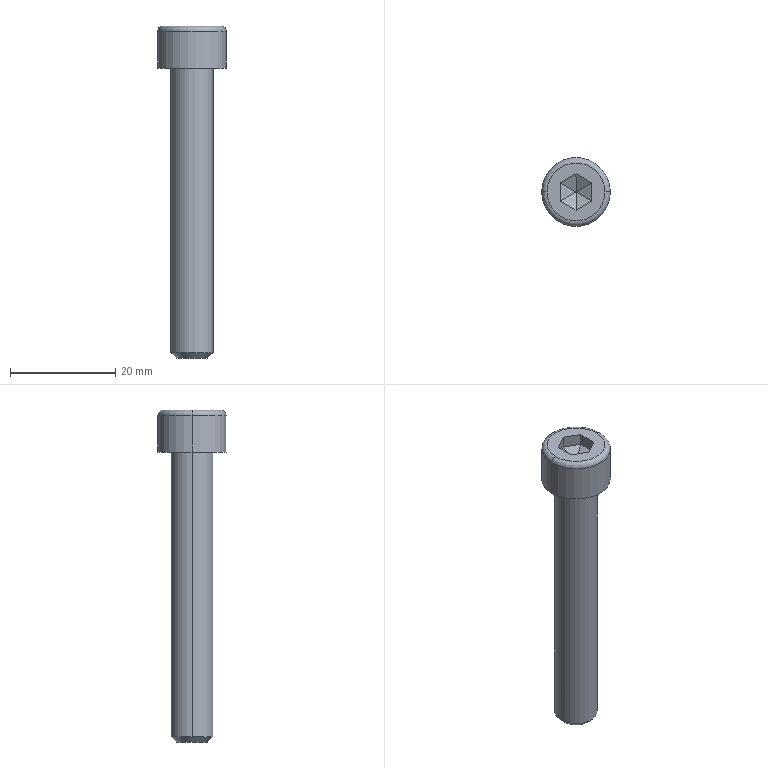Part | SolidWorks | features Chamfer 2, Fillet 2, ICE 2, Extrusion 1, RefAxis 1 | 1 solid | 26 faces | box 13 x 13 x 63 mm | volume 3718 mm3 | plane 16 | torus 4 | cylinder 4 | cone 2 | commonest cylinder face diameters 8 x2 13 x2
STEP:
#1=CARTESIAN_POINT('',(-4.1,0.,0.));
#2=VERTEX_POINT('',#1);
#3=CARTESIAN_POINT('',(4.1,0.,0.));
#4=VERTEX_POINT('',#3);
#5=CARTESIAN_POINT('',(0.,0.,0.));
#6=DIRECTION('',(0.,0.,1.));
#7=DIRECTION('',(1.,0.,0.));
#8=AXIS2_PLACEMENT_3D('',#5,#6,#7);
#9=CIRCLE('',#8,4.1);
#10=EDGE_CURVE('',#2,#4,#9,.T.);
#11=ORIENTED_EDGE('',*,*,#10,.F.);
#12=CARTESIAN_POINT('',(-4.,0.,-0.1));
#13=VERTEX_POINT('',#12);
#14=CARTESIAN_POINT('',(-4.1,0.,-0.1));
#15=DIRECTION('',(0.,1.,0.));
#16=DIRECTION('',(-1.,0.,0.));
#17=AXIS2_PLACEMENT_3D('',#14,#15,#16);
#18=CIRCLE('',#17,0.1);
#19=EDGE_CURVE('',#2,#13,#18,.T.);
#20=ORIENTED_EDGE('',*,*,#19,.T.);
#21=CARTESIAN_POINT('',(4.,0.,-0.1));
#22=VERTEX_POINT('',#21);
#23=CARTESIAN_POINT('',(0.,0.,-0.1));
#24=DIRECTION('',(0.,0.,-1.));
#25=DIRECTION('',(1.,0.,0.));
#26=AXIS2_PLACEMENT_3D('',#23,#24,#25);
#27=CIRCLE('',#26,4.);
#28=EDGE_CURVE('',#22,#13,#27,.T.);
#29=ORIENTED_EDGE('',*,*,#28,.F.);
#30=CARTESIAN_POINT('',(4.1,0.,-0.1));
#31=DIRECTION('',(0.,-1.,0.));
#32=DIRECTION('',(0.,0.,-1.));
#33=AXIS2_PLACEMENT_3D('',#30,#31,#32);
#34=CIRCLE('',#33,0.1);
#35=EDGE_CURVE('',#4,#22,#34,.T.);
#36=ORIENTED_EDGE('',*,*,#35,.F.);
#37=EDGE_LOOP('',(#11,#20,#29,#36));
#38=FACE_OUTER_BOUND('',#37,.T.);
#39=CARTESIAN_POINT('',(0.,0.,-0.1));
#40=DIRECTION('',(0.,0.,1.));
#41=DIRECTION('',(1.,0.,0.));
#42=AXIS2_PLACEMENT_3D('',#39,#40,#41);
#43=TOROIDAL_SURFACE('',#42,4.1,0.1);
#44=ADVANCED_FACE('',(#38),#43,.F.);
#45=CARTESIAN_POINT('',(-6.5,0.,7.));
#46=VERTEX_POINT('',#45);
#47=CARTESIAN_POINT('',(6.5,0.,7.));
#48=VERTEX_POINT('',#47);
#49=CARTESIAN_POINT('',(0.,0.,7.));
#50=DIRECTION('',(0.,0.,-1.));
#51=DIRECTION('',(1.,0.,0.));
#52=AXIS2_PLACEMENT_3D('',#49,#50,#51);
#53=CIRCLE('',#52,6.5);
#54=EDGE_CURVE('',#46,#48,#53,.T.);
#55=ORIENTED_EDGE('',*,*,#54,.F.);
#56=CARTESIAN_POINT('',(-5.5,0.,8.));
#57=VERTEX_POINT('',#56);
#58=CARTESIAN_POINT('',(-5.5,0.,7.));
#59=DIRECTION('',(0.,1.,0.));
#60=DIRECTION('',(-1.,0.,0.));
#61=AXIS2_PLACEMENT_3D('',#58,#59,#60);
#62=CIRCLE('',#61,1.);
#63=EDGE_CURVE('',#46,#57,#62,.T.);
#64=ORIENTED_EDGE('',*,*,#63,.T.);
#65=CARTESIAN_POINT('',(5.5,0.,8.));
#66=VERTEX_POINT('',#65);
#67=CARTESIAN_POINT('',(0.,0.,8.));
#68=DIRECTION('',(0.,0.,1.));
#69=DIRECTION('',(1.,0.,0.));
#70=AXIS2_PLACEMENT_3D('',#67,#68,#69);
#71=CIRCLE('',#70,5.5);
#72=EDGE_CURVE('',#66,#57,#71,.T.);
#73=ORIENTED_EDGE('',*,*,#72,.F.);
#74=CARTESIAN_POINT('',(5.5,0.,7.));
#75=DIRECTION('',(0.,-1.,0.));
#76=DIRECTION('',(0.,0.,-1.));
#77=AXIS2_PLACEMENT_3D('',#74,#75,#76);
#78=CIRCLE('',#77,1.);
#79=EDGE_CURVE('',#48,#66,#78,.T.);
#80=ORIENTED_EDGE('',*,*,#79,.F.);
#81=EDGE_LOOP('',(#55,#64,#73,#80));
#82=FACE_OUTER_BOUND('',#81,.T.);
#83=CARTESIAN_POINT('',(0.,0.,7.));
#84=DIRECTION('',(0.,0.,1.));
#85=DIRECTION('',(1.,0.,0.));
#86=AXIS2_PLACEMENT_3D('',#83,#84,#85);
#87=TOROIDAL_SURFACE('',#86,5.5,1.);
#88=ADVANCED_FACE('',(#82),#87,.T.);
#89=CARTESIAN_POINT('',(-3.,0.,-55.));
#90=VERTEX_POINT('',#89);
#91=CARTESIAN_POINT('',(3.,0.,-55.));
#92=VERTEX_POINT('',#91);
#93=CARTESIAN_POINT('',(0.,0.,-55.));
#94=DIRECTION('',(0.,0.,-1.));
#95=DIRECTION('',(-1.,0.,0.));
#96=AXIS2_PLACEMENT_3D('',#93,#94,#95);
#97=CIRCLE('',#96,3.);
#98=EDGE_CURVE('',#90,#92,#97,.T.);
#99=ORIENTED_EDGE('',*,*,#98,.F.);
#100=CARTESIAN_POINT('',(-4.,0.,-54.));
#101=VERTEX_POINT('',#100);
#102=CARTESIAN_POINT('',(-3.,0.,-55.));
#103=DIRECTION('',(-0.7071,0.,0.7071));
#104=VECTOR('',#103,1000.);
#105=LINE('',#102,#104);
#106=EDGE_CURVE('',#90,#101,#105,.T.);
#107=ORIENTED_EDGE('',*,*,#106,.T.);
#108=CARTESIAN_POINT('',(4.,0.,-54.));
#109=VERTEX_POINT('',#108);
#110=CARTESIAN_POINT('',(0.,0.,-54.));
#111=DIRECTION('',(0.,0.,1.));
#112=DIRECTION('',(-1.,0.,0.));
#113=AXIS2_PLACEMENT_3D('',#110,#111,#112);
#114=CIRCLE('',#113,4.);
#115=EDGE_CURVE('',#109,#101,#114,.T.);
#116=ORIENTED_EDGE('',*,*,#115,.F.);
#117=CARTESIAN_POINT('',(3.,0.,-55.));
#118=DIRECTION('',(0.7071,0.,0.7071));
#119=VECTOR('',#118,1000.);
#120=LINE('',#117,#119);
#121=EDGE_CURVE('',#92,#109,#120,.T.);
#122=ORIENTED_EDGE('',*,*,#121,.F.);
#123=EDGE_LOOP('',(#99,#107,#116,#122));
#124=FACE_OUTER_BOUND('',#123,.T.);
#125=CARTESIAN_POINT('',(0.,0.,-55.));
#126=DIRECTION('',(0.,0.,1.));
#127=DIRECTION('',(1.,0.,0.));
#128=AXIS2_PLACEMENT_3D('',#125,#126,#127);
#129=CONICAL_SURFACE('',#128,3.,0.7854);
#130=ADVANCED_FACE('',(#124),#129,.T.);
#131=ORIENTED_EDGE('',*,*,#115,.T.);
#132=CARTESIAN_POINT('',(-4.,0.,-55.));
#133=DIRECTION('',(0.,0.,1.));
#134=VECTOR('',#133,1000.);
#135=LINE('',#132,#134);
#136=EDGE_CURVE('',#101,#13,#135,.T.);
#137=ORIENTED_EDGE('',*,*,#136,.T.);
#138=CARTESIAN_POINT('',(0.,0.,-0.1));
#139=DIRECTION('',(0.,0.,-1.));
#140=DIRECTION('',(1.,0.,0.));
#141=AXIS2_PLACEMENT_3D('',#138,#139,#140);
#142=CIRCLE('',#141,4.);
#143=EDGE_CURVE('',#13,#22,#142,.T.);
#144=ORIENTED_EDGE('',*,*,#143,.T.);
#145=CARTESIAN_POINT('',(4.,0.,-55.));
#146=DIRECTION('',(0.,0.,1.));
#147=VECTOR('',#146,1000.);
#148=LINE('',#145,#147);
#149=EDGE_CURVE('',#109,#22,#148,.T.);
#150=ORIENTED_EDGE('',*,*,#149,.F.);
#151=EDGE_LOOP('',(#131,#137,#144,#150));
#152=FACE_OUTER_BOUND('',#151,.T.);
#153=CARTESIAN_POINT('',(0.,0.,-55.));
#154=DIRECTION('',(0.,0.,1.));
#155=DIRECTION('',(1.,0.,0.));
#156=AXIS2_PLACEMENT_3D('',#153,#154,#155);
#157=CYLINDRICAL_SURFACE('',#156,4.);
#158=ADVANCED_FACE('',(#152),#157,.T.);
#159=ORIENTED_EDGE('',*,*,#54,.T.);
#160=CARTESIAN_POINT('',(6.5,0.,0.));
#161=VERTEX_POINT('',#160);
#162=CARTESIAN_POINT('',(6.5,0.,8.));
#163=DIRECTION('',(0.,0.,-1.));
#164=VECTOR('',#163,1000.);
#165=LINE('',#162,#164);
#166=EDGE_CURVE('',#48,#161,#165,.T.);
#167=ORIENTED_EDGE('',*,*,#166,.T.);
#168=CARTESIAN_POINT('',(-6.5,0.,0.));
#169=VERTEX_POINT('',#168);
#170=CARTESIAN_POINT('',(0.,0.,0.));
#171=DIRECTION('',(0.,0.,1.));
#172=DIRECTION('',(1.,0.,0.));
#173=AXIS2_PLACEMENT_3D('',#170,#171,#172);
#174=CIRCLE('',#173,6.5);
#175=EDGE_CURVE('',#161,#169,#174,.T.);
#176=ORIENTED_EDGE('',*,*,#175,.T.);
#177=CARTESIAN_POINT('',(-6.5,0.,8.));
#178=DIRECTION('',(0.,0.,-1.));
#179=VECTOR('',#178,1000.);
#180=LINE('',#177,#179);
#181=EDGE_CURVE('',#46,#169,#180,.T.);
#182=ORIENTED_EDGE('',*,*,#181,.F.);
#183=EDGE_LOOP('',(#159,#167,#176,#182));
#184=FACE_OUTER_BOUND('',#183,.T.);
#185=CARTESIAN_POINT('',(0.,0.,8.));
#186=DIRECTION('',(0.,0.,-1.));
#187=DIRECTION('',(-1.,0.,0.));
#188=AXIS2_PLACEMENT_3D('',#185,#186,#187);
#189=CYLINDRICAL_SURFACE('',#188,6.5);
#190=ADVANCED_FACE('',(#184),#189,.T.);
#191=CARTESIAN_POINT('',(0.,0.,0.));
#192=DIRECTION('',(0.,0.,1.));
#193=DIRECTION('',(1.,0.,0.));
#194=AXIS2_PLACEMENT_3D('',#191,#192,#193);
#195=CIRCLE('',#194,4.1);
#196=EDGE_CURVE('',#4,#2,#195,.T.);
#197=ORIENTED_EDGE('',*,*,#196,.T.);
#198=ORIENTED_EDGE('',*,*,#10,.T.);
#199=EDGE_LOOP('',(#197,#198));
#200=FACE_BOUND('',#199,.T.);
#201=CARTESIAN_POINT('',(0.,0.,0.));
#202=DIRECTION('',(0.,0.,1.));
#203=DIRECTION('',(1.,0.,0.));
#204=AXIS2_PLACEMENT_3D('',#201,#202,#203);
#205=CIRCLE('',#204,6.5);
#206=EDGE_CURVE('',#169,#161,#205,.T.);
#207=ORIENTED_EDGE('',*,*,#206,.F.);
#208=ORIENTED_EDGE('',*,*,#175,.F.);
#209=EDGE_LOOP('',(#207,#208));
#210=FACE_OUTER_BOUND('',#209,.T.);
#211=CARTESIAN_POINT('',(0.,0.,0.));
#212=DIRECTION('',(0.,0.,1.));
#213=DIRECTION('',(1.,0.,0.));
#214=AXIS2_PLACEMENT_3D('',#211,#212,#213);
#215=PLANE('',#214);
#216=ADVANCED_FACE('',(#200,#210),#215,.F.);
#217=ORIENTED_EDGE('',*,*,#166,.F.);
#218=CARTESIAN_POINT('',(0.,0.,7.));
#219=DIRECTION('',(0.,0.,-1.));
#220=DIRECTION('',(1.,0.,0.));
#221=AXIS2_PLACEMENT_3D('',#218,#219,#220);
#222=CIRCLE('',#221,6.5);
#223=EDGE_CURVE('',#48,#46,#222,.T.);
#224=ORIENTED_EDGE('',*,*,#223,.T.);
#225=ORIENTED_EDGE('',*,*,#181,.T.);
#226=ORIENTED_EDGE('',*,*,#206,.T.);
#227=EDGE_LOOP('',(#217,#224,#225,#226));
#228=FACE_OUTER_BOUND('',#227,.T.);
#229=CARTESIAN_POINT('',(0.,0.,8.));
#230=DIRECTION('',(0.,0.,-1.));
#231=DIRECTION('',(-1.,0.,0.));
#232=AXIS2_PLACEMENT_3D('',#229,#230,#231);
#233=CYLINDRICAL_SURFACE('',#232,6.5);
#234=ADVANCED_FACE('',(#228),#233,.T.);
#235=ORIENTED_EDGE('',*,*,#72,.T.);
#236=CARTESIAN_POINT('',(0.,0.,8.));
#237=DIRECTION('',(0.,0.,1.));
#238=DIRECTION('',(1.,0.,0.));
#239=AXIS2_PLACEMENT_3D('',#236,#237,#238);
#240=CIRCLE('',#239,5.5);
#241=EDGE_CURVE('',#57,#66,#240,.T.);
#242=ORIENTED_EDGE('',*,*,#241,.T.);
#243=EDGE_LOOP('',(#235,#242));
#244=FACE_OUTER_BOUND('',#243,.T.);
#245=CARTESIAN_POINT('',(3.,-1.732,8.));
#246=VERTEX_POINT('',#245);
#247=CARTESIAN_POINT('',(3.,1.732,8.));
#248=VERTEX_POINT('',#247);
#249=CARTESIAN_POINT('',(3.,-1.732,8.));
#250=DIRECTION('',(0.,1.,0.));
#251=VECTOR('',#250,1000.);
#252=LINE('',#249,#251);
#253=EDGE_CURVE('',#246,#248,#252,.T.);
#254=ORIENTED_EDGE('',*,*,#253,.F.);
#255=CARTESIAN_POINT('',(0.,-3.464,8.));
#256=VERTEX_POINT('',#255);
#257=CARTESIAN_POINT('',(0.,-3.464,8.));
#258=DIRECTION('',(0.866,0.5,0.));
#259=VECTOR('',#258,1000.);
#260=LINE('',#257,#259);
#261=EDGE_CURVE('',#256,#246,#260,.T.);
#262=ORIENTED_EDGE('',*,*,#261,.F.);
#263=CARTESIAN_POINT('',(-3.,-1.732,8.));
#264=VERTEX_POINT('',#263);
#265=CARTESIAN_POINT('',(-3.,-1.732,8.));
#266=DIRECTION('',(0.866,-0.5,0.));
#267=VECTOR('',#266,1000.);
#268=LINE('',#265,#267);
#269=EDGE_CURVE('',#264,#256,#268,.T.);
#270=ORIENTED_EDGE('',*,*,#269,.F.);
#271=CARTESIAN_POINT('',(-3.,1.732,8.));
#272=VERTEX_POINT('',#271);
#273=CARTESIAN_POINT('',(-3.,1.732,8.));
#274=DIRECTION('',(0.,-1.,0.));
#275=VECTOR('',#274,1000.);
#276=LINE('',#273,#275);
#277=EDGE_CURVE('',#272,#264,#276,.T.);
#278=ORIENTED_EDGE('',*,*,#277,.F.);
#279=CARTESIAN_POINT('',(0.,3.464,8.));
#280=VERTEX_POINT('',#279);
#281=CARTESIAN_POINT('',(0.,3.464,8.));
#282=DIRECTION('',(-0.866,-0.5,0.));
#283=VECTOR('',#282,1000.);
#284=LINE('',#281,#283);
#285=EDGE_CURVE('',#280,#272,#284,.T.);
#286=ORIENTED_EDGE('',*,*,#285,.F.);
#287=CARTESIAN_POINT('',(3.,1.732,8.));
#288=DIRECTION('',(-0.866,0.5,0.));
#289=VECTOR('',#288,1000.);
#290=LINE('',#287,#289);
#291=EDGE_CURVE('',#248,#280,#290,.T.);
#292=ORIENTED_EDGE('',*,*,#291,.F.);
#293=EDGE_LOOP('',(#254,#262,#270,#278,#286,#292));
#294=FACE_BOUND('',#293,.T.);
#295=CARTESIAN_POINT('',(0.,0.,8.));
#296=DIRECTION('',(0.,0.,1.));
#297=DIRECTION('',(1.,0.,0.));
#298=AXIS2_PLACEMENT_3D('',#295,#296,#297);
#299=PLANE('',#298);
#300=ADVANCED_FACE('',(#244,#294),#299,.T.);
#301=CARTESIAN_POINT('',(3.,1.732,5.729));
#302=VERTEX_POINT('',#301);
#303=CARTESIAN_POINT('',(3.,1.732,4.));
#304=DIRECTION('',(0.,0.,1.));
#305=VECTOR('',#304,1000.);
#306=LINE('',#303,#305);
#307=EDGE_CURVE('',#302,#248,#306,.T.);
#308=ORIENTED_EDGE('',*,*,#307,.F.);
#309=CARTESIAN_POINT('',(3.,-1.732,5.729));
#310=VERTEX_POINT('',#309);
#311=CARTESIAN_POINT('',(3.,-1.732,5.729));
#312=DIRECTION('',(0.,-1.,0.));
#313=VECTOR('',#312,1000.);
#314=LINE('',#311,#313);
#315=EDGE_CURVE('',#302,#310,#314,.T.);
#316=ORIENTED_EDGE('',*,*,#315,.T.);
#317=CARTESIAN_POINT('',(3.,-1.732,4.));
#318=DIRECTION('',(0.,0.,1.));
#319=VECTOR('',#318,1000.);
#320=LINE('',#317,#319);
#321=EDGE_CURVE('',#310,#246,#320,.T.);
#322=ORIENTED_EDGE('',*,*,#321,.T.);
#323=ORIENTED_EDGE('',*,*,#253,.T.);
#324=EDGE_LOOP('',(#308,#316,#322,#323));
#325=FACE_OUTER_BOUND('',#324,.T.);
#326=CARTESIAN_POINT('',(3.,-1.732,4.));
#327=DIRECTION('',(1.,0.,0.));
#328=DIRECTION('',(0.,1.,0.));
#329=AXIS2_PLACEMENT_3D('',#326,#327,#328);
#330=PLANE('',#329);
#331=ADVANCED_FACE('',(#325),#330,.F.);
#332=ORIENTED_EDGE('',*,*,#321,.F.);
#333=CARTESIAN_POINT('',(0.,-3.464,5.729));
#334=VERTEX_POINT('',#333);
#335=CARTESIAN_POINT('',(0.,-3.464,5.729));
#336=DIRECTION('',(-0.866,-0.5,0.));
#337=VECTOR('',#336,1000.);
#338=LINE('',#335,#337);
#339=EDGE_CURVE('',#310,#334,#338,.T.);
#340=ORIENTED_EDGE('',*,*,#339,.T.);
#341=CARTESIAN_POINT('',(0.,-3.464,4.));
#342=DIRECTION('',(0.,0.,1.));
#343=VECTOR('',#342,1000.);
#344=LINE('',#341,#343);
#345=EDGE_CURVE('',#334,#256,#344,.T.);
#346=ORIENTED_EDGE('',*,*,#345,.T.);
#347=ORIENTED_EDGE('',*,*,#261,.T.);
#348=EDGE_LOOP('',(#332,#340,#346,#347));
#349=FACE_OUTER_BOUND('',#348,.T.);
#350=CARTESIAN_POINT('',(0.,-3.464,4.));
#351=DIRECTION('',(0.5,-0.866,0.));
#352=DIRECTION('',(0.866,0.5,0.));
#353=AXIS2_PLACEMENT_3D('',#350,#351,#352);
#354=PLANE('',#353);
#355=ADVANCED_FACE('',(#349),#354,.F.);
#356=ORIENTED_EDGE('',*,*,#345,.F.);
#357=CARTESIAN_POINT('',(-3.,-1.732,5.729));
#358=VERTEX_POINT('',#357);
#359=CARTESIAN_POINT('',(-3.,-1.732,5.729));
#360=DIRECTION('',(-0.866,0.5,0.));
#361=VECTOR('',#360,1000.);
#362=LINE('',#359,#361);
#363=EDGE_CURVE('',#334,#358,#362,.T.);
#364=ORIENTED_EDGE('',*,*,#363,.T.);
#365=CARTESIAN_POINT('',(-3.,-1.732,4.));
#366=DIRECTION('',(0.,0.,1.));
#367=VECTOR('',#366,1000.);
#368=LINE('',#365,#367);
#369=EDGE_CURVE('',#358,#264,#368,.T.);
#370=ORIENTED_EDGE('',*,*,#369,.T.);
#371=ORIENTED_EDGE('',*,*,#269,.T.);
#372=EDGE_LOOP('',(#356,#364,#370,#371));
#373=FACE_OUTER_BOUND('',#372,.T.);
#374=CARTESIAN_POINT('',(-3.,-1.732,4.));
#375=DIRECTION('',(-0.5,-0.866,0.));
#376=DIRECTION('',(0.866,-0.5,0.));
#377=AXIS2_PLACEMENT_3D('',#374,#375,#376);
#378=PLANE('',#377);
#379=ADVANCED_FACE('',(#373),#378,.F.);
#380=ORIENTED_EDGE('',*,*,#369,.F.);
#381=CARTESIAN_POINT('',(-3.,1.732,5.729));
#382=VERTEX_POINT('',#381);
#383=CARTESIAN_POINT('',(-3.,1.732,5.729));
#384=DIRECTION('',(0.,1.,0.));
#385=VECTOR('',#384,1000.);
#386=LINE('',#383,#385);
#387=EDGE_CURVE('',#358,#382,#386,.T.);
#388=ORIENTED_EDGE('',*,*,#387,.T.);
#389=CARTESIAN_POINT('',(-3.,1.732,4.));
#390=DIRECTION('',(0.,0.,1.));
#391=VECTOR('',#390,1000.);
#392=LINE('',#389,#391);
#393=EDGE_CURVE('',#382,#272,#392,.T.);
#394=ORIENTED_EDGE('',*,*,#393,.T.);
#395=ORIENTED_EDGE('',*,*,#277,.T.);
#396=EDGE_LOOP('',(#380,#388,#394,#395));
#397=FACE_OUTER_BOUND('',#396,.T.);
#398=CARTESIAN_POINT('',(-3.,1.732,4.));
#399=DIRECTION('',(-1.,0.,0.));
#400=DIRECTION('',(0.,0.,1.));
#401=AXIS2_PLACEMENT_3D('',#398,#399,#400);
#402=PLANE('',#401);
#403=ADVANCED_FACE('',(#397),#402,.F.);
#404=ORIENTED_EDGE('',*,*,#393,.F.);
#405=CARTESIAN_POINT('',(0.,3.464,5.729));
#406=VERTEX_POINT('',#405);
#407=CARTESIAN_POINT('',(0.,3.464,5.729));
#408=DIRECTION('',(0.866,0.5,0.));
#409=VECTOR('',#408,1000.);
#410=LINE('',#407,#409);
#411=EDGE_CURVE('',#382,#406,#410,.T.);
#412=ORIENTED_EDGE('',*,*,#411,.T.);
#413=CARTESIAN_POINT('',(0.,3.464,4.));
#414=DIRECTION('',(0.,0.,1.));
#415=VECTOR('',#414,1000.);
#416=LINE('',#413,#415);
#417=EDGE_CURVE('',#406,#280,#416,.T.);
#418=ORIENTED_EDGE('',*,*,#417,.T.);
#419=ORIENTED_EDGE('',*,*,#285,.T.);
#420=EDGE_LOOP('',(#404,#412,#418,#419));
#421=FACE_OUTER_BOUND('',#420,.T.);
#422=CARTESIAN_POINT('',(0.,3.464,4.));
#423=DIRECTION('',(-0.5,0.866,0.));
#424=DIRECTION('',(-0.866,-0.5,0.));
#425=AXIS2_PLACEMENT_3D('',#422,#423,#424);
#426=PLANE('',#425);
#427=ADVANCED_FACE('',(#421),#426,.F.);
#428=ORIENTED_EDGE('',*,*,#417,.F.);
#429=CARTESIAN_POINT('',(3.,1.732,5.729));
#430=DIRECTION('',(0.866,-0.5,0.));
#431=VECTOR('',#430,1000.);
#432=LINE('',#429,#431);
#433=EDGE_CURVE('',#406,#302,#432,.T.);
#434=ORIENTED_EDGE('',*,*,#433,.T.);
#435=ORIENTED_EDGE('',*,*,#307,.T.);
#436=ORIENTED_EDGE('',*,*,#291,.T.);
#437=EDGE_LOOP('',(#428,#434,#435,#436));
#438=FACE_OUTER_BOUND('',#437,.T.);
#439=CARTESIAN_POINT('',(3.,1.732,4.));
#440=DIRECTION('',(0.5,0.866,0.));
#441=DIRECTION('',(-0.866,0.5,0.));
#442=AXIS2_PLACEMENT_3D('',#439,#440,#441);
#443=PLANE('',#442);
#444=ADVANCED_FACE('',(#438),#443,.F.);
#445=CARTESIAN_POINT('',(0.,0.005888,4.));
#446=VERTEX_POINT('',#445);
#447=CARTESIAN_POINT('',(-0.005099,0.002944,4.));
#448=VERTEX_POINT('',#447);
#449=CARTESIAN_POINT('',(-0.00255,0.004416,4.));
#450=DIRECTION('',(-0.866,-0.5,0.));
#451=VECTOR('',#450,1000.);
#452=LINE('',#449,#451);
#453=EDGE_CURVE('',#446,#448,#452,.T.);
#454=ORIENTED_EDGE('',*,*,#453,.T.);
#455=CARTESIAN_POINT('',(-0.005099,-0.002944,4.));
#456=VERTEX_POINT('',#455);
#457=CARTESIAN_POINT('',(-0.005099,0.,4.));
#458=DIRECTION('',(0.,-1.,0.));
#459=VECTOR('',#458,1000.);
#460=LINE('',#457,#459);
#461=EDGE_CURVE('',#448,#456,#460,.T.);
#462=ORIENTED_EDGE('',*,*,#461,.T.);
#463=CARTESIAN_POINT('',(0.,-0.005888,4.));
#464=VERTEX_POINT('',#463);
#465=CARTESIAN_POINT('',(-0.00255,-0.004416,4.));
#466=DIRECTION('',(0.866,-0.5,0.));
#467=VECTOR('',#466,1000.);
#468=LINE('',#465,#467);
#469=EDGE_CURVE('',#456,#464,#468,.T.);
#470=ORIENTED_EDGE('',*,*,#469,.T.);
#471=CARTESIAN_POINT('',(0.005099,-0.002944,4.));
#472=VERTEX_POINT('',#471);
#473=CARTESIAN_POINT('',(0.00255,-0.004416,4.));
#474=DIRECTION('',(0.866,0.5,0.));
#475=VECTOR('',#474,1000.);
#476=LINE('',#473,#475);
#477=EDGE_CURVE('',#464,#472,#476,.T.);
#478=ORIENTED_EDGE('',*,*,#477,.T.);
#479=CARTESIAN_POINT('',(0.005099,0.002944,4.));
#480=VERTEX_POINT('',#479);
#481=CARTESIAN_POINT('',(0.005099,0.,4.));
#482=DIRECTION('',(0.,1.,0.));
#483=VECTOR('',#482,1000.);
#484=LINE('',#481,#483);
#485=EDGE_CURVE('',#472,#480,#484,.T.);
#486=ORIENTED_EDGE('',*,*,#485,.T.);
#487=CARTESIAN_POINT('',(0.00255,0.004416,4.));
#488=DIRECTION('',(-0.866,0.5,0.));
#489=VECTOR('',#488,1000.);
#490=LINE('',#487,#489);
#491=EDGE_CURVE('',#480,#446,#490,.T.);
#492=ORIENTED_EDGE('',*,*,#491,.T.);
#493=EDGE_LOOP('',(#454,#462,#470,#478,#486,#492));
#494=FACE_OUTER_BOUND('',#493,.T.);
#495=CARTESIAN_POINT('',(0.,0.,4.));
#496=DIRECTION('',(0.,0.,1.));
#497=DIRECTION('',(1.,0.,0.));
#498=AXIS2_PLACEMENT_3D('',#495,#496,#497);
#499=PLANE('',#498);
#500=ADVANCED_FACE('',(#494),#499,.T.);
#501=ORIENTED_EDGE('',*,*,#136,.F.);
#502=CARTESIAN_POINT('',(0.,0.,-54.));
#503=DIRECTION('',(0.,0.,1.));
#504=DIRECTION('',(-1.,0.,0.));
#505=AXIS2_PLACEMENT_3D('',#502,#503,#504);
#506=CIRCLE('',#505,4.);
#507=EDGE_CURVE('',#101,#109,#506,.T.);
#508=ORIENTED_EDGE('',*,*,#507,.T.);
#509=ORIENTED_EDGE('',*,*,#149,.T.);
#510=ORIENTED_EDGE('',*,*,#28,.T.);
#511=EDGE_LOOP('',(#501,#508,#509,#510));
#512=FACE_OUTER_BOUND('',#511,.T.);
#513=CARTESIAN_POINT('',(0.,0.,-55.));
#514=DIRECTION('',(0.,0.,1.));
#515=DIRECTION('',(1.,0.,0.));
#516=AXIS2_PLACEMENT_3D('',#513,#514,#515);
#517=CYLINDRICAL_SURFACE('',#516,4.);
#518=ADVANCED_FACE('',(#512),#517,.T.);
#519=CARTESIAN_POINT('',(0.,0.,-55.));
#520=DIRECTION('',(0.,0.,-1.));
#521=DIRECTION('',(-1.,0.,0.));
#522=AXIS2_PLACEMENT_3D('',#519,#520,#521);
#523=CIRCLE('',#522,3.);
#524=EDGE_CURVE('',#92,#90,#523,.T.);
#525=ORIENTED_EDGE('',*,*,#524,.T.);
#526=ORIENTED_EDGE('',*,*,#98,.T.);
#527=EDGE_LOOP('',(#525,#526));
#528=FACE_OUTER_BOUND('',#527,.T.);
#529=CARTESIAN_POINT('',(0.,0.,-55.));
#530=DIRECTION('',(0.,0.,-1.));
#531=DIRECTION('',(-1.,0.,0.));
#532=AXIS2_PLACEMENT_3D('',#529,#530,#531);
#533=PLANE('',#532);
#534=ADVANCED_FACE('',(#528),#533,.T.);
#535=ORIENTED_EDGE('',*,*,#106,.F.);
#536=ORIENTED_EDGE('',*,*,#524,.F.);
#537=ORIENTED_EDGE('',*,*,#121,.T.);
#538=ORIENTED_EDGE('',*,*,#507,.F.);
#539=EDGE_LOOP('',(#535,#536,#537,#538));
#540=FACE_OUTER_BOUND('',#539,.T.);
#541=CARTESIAN_POINT('',(0.,0.,-55.));
#542=DIRECTION('',(0.,0.,1.));
#543=DIRECTION('',(1.,0.,0.));
#544=AXIS2_PLACEMENT_3D('',#541,#542,#543);
#545=CONICAL_SURFACE('',#544,3.,0.7854);
#546=ADVANCED_FACE('',(#540),#545,.T.);
#547=ORIENTED_EDGE('',*,*,#63,.F.);
#548=ORIENTED_EDGE('',*,*,#223,.F.);
#549=ORIENTED_EDGE('',*,*,#79,.T.);
#550=ORIENTED_EDGE('',*,*,#241,.F.);
#551=EDGE_LOOP('',(#547,#548,#549,#550));
#552=FACE_OUTER_BOUND('',#551,.T.);
#553=CARTESIAN_POINT('',(0.,0.,7.));
#554=DIRECTION('',(0.,0.,1.));
#555=DIRECTION('',(1.,0.,0.));
#556=AXIS2_PLACEMENT_3D('',#553,#554,#555);
#557=TOROIDAL_SURFACE('',#556,5.5,1.);
#558=ADVANCED_FACE('',(#552),#557,.T.);
#559=CARTESIAN_POINT('',(0.00408,-0.002355,3.999));
#560=DIRECTION('',(-0.7746,0.4472,-0.4472));
#561=VECTOR('',#560,1000.);
#562=LINE('',#559,#561);
#563=EDGE_CURVE('',#310,#472,#562,.T.);
#564=ORIENTED_EDGE('',*,*,#563,.F.);
#565=ORIENTED_EDGE('',*,*,#315,.F.);
#566=CARTESIAN_POINT('',(0.00408,0.002355,3.999));
#567=DIRECTION('',(0.7746,0.4472,0.4472));
#568=VECTOR('',#567,1000.);
#569=LINE('',#566,#568);
#570=EDGE_CURVE('',#480,#302,#569,.T.);
#571=ORIENTED_EDGE('',*,*,#570,.F.);
#572=ORIENTED_EDGE('',*,*,#485,.F.);
#573=EDGE_LOOP('',(#564,#565,#571,#572));
#574=FACE_OUTER_BOUND('',#573,.T.);
#575=CARTESIAN_POINT('',(0.005099,0.,4.));
#576=DIRECTION('',(0.5,0.,-0.866));
#577=DIRECTION('',(0.,1.,0.));
#578=AXIS2_PLACEMENT_3D('',#575,#576,#577);
#579=PLANE('',#578);
#580=ADVANCED_FACE('',(#574),#579,.F.);
#581=ORIENTED_EDGE('',*,*,#570,.T.);
#582=ORIENTED_EDGE('',*,*,#433,.F.);
#583=CARTESIAN_POINT('',(0.,0.004711,3.999));
#584=DIRECTION('',(0.,0.8944,0.4472));
#585=VECTOR('',#584,1000.);
#586=LINE('',#583,#585);
#587=EDGE_CURVE('',#446,#406,#586,.T.);
#588=ORIENTED_EDGE('',*,*,#587,.F.);
#589=ORIENTED_EDGE('',*,*,#491,.F.);
#590=EDGE_LOOP('',(#581,#582,#588,#589));
#591=FACE_OUTER_BOUND('',#590,.T.);
#592=CARTESIAN_POINT('',(0.00255,0.004416,4.));
#593=DIRECTION('',(0.25,0.433,-0.866));
#594=DIRECTION('',(-0.866,0.5,0.));
#595=AXIS2_PLACEMENT_3D('',#592,#593,#594);
#596=PLANE('',#595);
#597=ADVANCED_FACE('',(#591),#596,.F.);
#598=ORIENTED_EDGE('',*,*,#563,.T.);
#599=ORIENTED_EDGE('',*,*,#477,.F.);
#600=CARTESIAN_POINT('',(0.,-0.004711,3.999));
#601=DIRECTION('',(0.,0.8944,-0.4472));
#602=VECTOR('',#601,1000.);
#603=LINE('',#600,#602);
#604=EDGE_CURVE('',#334,#464,#603,.T.);
#605=ORIENTED_EDGE('',*,*,#604,.F.);
#606=ORIENTED_EDGE('',*,*,#339,.F.);
#607=EDGE_LOOP('',(#598,#599,#605,#606));
#608=FACE_OUTER_BOUND('',#607,.T.);
#609=CARTESIAN_POINT('',(0.00255,-0.004416,4.));
#610=DIRECTION('',(0.25,-0.433,-0.866));
#611=DIRECTION('',(0.866,0.5,0.));
#612=AXIS2_PLACEMENT_3D('',#609,#610,#611);
#613=PLANE('',#612);
#614=ADVANCED_FACE('',(#608),#613,.F.);
#615=ORIENTED_EDGE('',*,*,#587,.T.);
#616=ORIENTED_EDGE('',*,*,#411,.F.);
#617=CARTESIAN_POINT('',(-0.00408,0.002355,3.999));
#618=DIRECTION('',(-0.7746,0.4472,0.4472));
#619=VECTOR('',#618,1000.);
#620=LINE('',#617,#619);
#621=EDGE_CURVE('',#448,#382,#620,.T.);
#622=ORIENTED_EDGE('',*,*,#621,.F.);
#623=ORIENTED_EDGE('',*,*,#453,.F.);
#624=EDGE_LOOP('',(#615,#616,#622,#623));
#625=FACE_OUTER_BOUND('',#624,.T.);
#626=CARTESIAN_POINT('',(-0.00255,0.004416,4.));
#627=DIRECTION('',(-0.25,0.433,-0.866));
#628=DIRECTION('',(-0.866,-0.5,0.));
#629=AXIS2_PLACEMENT_3D('',#626,#627,#628);
#630=PLANE('',#629);
#631=ADVANCED_FACE('',(#625),#630,.F.);
#632=ORIENTED_EDGE('',*,*,#604,.T.);
#633=ORIENTED_EDGE('',*,*,#469,.F.);
#634=CARTESIAN_POINT('',(-0.00408,-0.002355,3.999));
#635=DIRECTION('',(0.7746,0.4472,-0.4472));
#636=VECTOR('',#635,1000.);
#637=LINE('',#634,#636);
#638=EDGE_CURVE('',#358,#456,#637,.T.);
#639=ORIENTED_EDGE('',*,*,#638,.F.);
#640=ORIENTED_EDGE('',*,*,#363,.F.);
#641=EDGE_LOOP('',(#632,#633,#639,#640));
#642=FACE_OUTER_BOUND('',#641,.T.);
#643=CARTESIAN_POINT('',(-0.00255,-0.004416,4.));
#644=DIRECTION('',(-0.25,-0.433,-0.866));
#645=DIRECTION('',(0.866,-0.5,0.));
#646=AXIS2_PLACEMENT_3D('',#643,#644,#645);
#647=PLANE('',#646);
#648=ADVANCED_FACE('',(#642),#647,.F.);
#649=ORIENTED_EDGE('',*,*,#621,.T.);
#650=ORIENTED_EDGE('',*,*,#387,.F.);
#651=ORIENTED_EDGE('',*,*,#638,.T.);
#652=ORIENTED_EDGE('',*,*,#461,.F.);
#653=EDGE_LOOP('',(#649,#650,#651,#652));
#654=FACE_OUTER_BOUND('',#653,.T.);
#655=CARTESIAN_POINT('',(-0.005099,0.,4.));
#656=DIRECTION('',(-0.5,0.,-0.866));
#657=DIRECTION('',(0.,-1.,0.));
#658=AXIS2_PLACEMENT_3D('',#655,#656,#657);
#659=PLANE('',#658);
#660=ADVANCED_FACE('',(#654),#659,.F.);
#661=ORIENTED_EDGE('',*,*,#19,.F.);
#662=ORIENTED_EDGE('',*,*,#196,.F.);
#663=ORIENTED_EDGE('',*,*,#35,.T.);
#664=ORIENTED_EDGE('',*,*,#143,.F.);
#665=EDGE_LOOP('',(#661,#662,#663,#664));
#666=FACE_OUTER_BOUND('',#665,.T.);
#667=CARTESIAN_POINT('',(0.,0.,-0.1));
#668=DIRECTION('',(0.,0.,1.));
#669=DIRECTION('',(1.,0.,0.));
#670=AXIS2_PLACEMENT_3D('',#667,#668,#669);
#671=TOROIDAL_SURFACE('',#670,4.1,0.1);
#672=ADVANCED_FACE('',(#666),#671,.F.);
#673=CLOSED_SHELL('',(#44,#88,#130,#158,#190,#216,#234,#300,#331,#355,#379,#403,#427,#444,#500,#518,#534,#546,#558,#580,#597,#614,#631,#648,#660,#672));
#674=MANIFOLD_SOLID_BREP('',#673);
#675=CARTESIAN_POINT('',(0.,0.,0.));
#676=DIRECTION('',(0.,0.,1.));
#677=DIRECTION('',(1.,0.,0.));
#678=AXIS2_PLACEMENT_3D('',#675,#676,#677);
#679=(LENGTH_UNIT()NAMED_UNIT(*)SI_UNIT(.MILLI.,.METRE.));
#680=UNCERTAINTY_MEASURE_WITH_UNIT(LENGTH_MEASURE(0.00001),#679,'','');
#681=(NAMED_UNIT(*)PLANE_ANGLE_UNIT()SI_UNIT($,.RADIAN.));
#682=(NAMED_UNIT(*)SI_UNIT($,.STERADIAN.)SOLID_ANGLE_UNIT());
#683=(GEOMETRIC_REPRESENTATION_CONTEXT(3)GLOBAL_UNCERTAINTY_ASSIGNED_CONTEXT((#680))GLOBAL_UNIT_ASSIGNED_CONTEXT((#679,#681,#682))REPRESENTATION_CONTEXT('',''));
#684=ADVANCED_BREP_SHAPE_REPRESENTATION('',(#674,#678),#683);